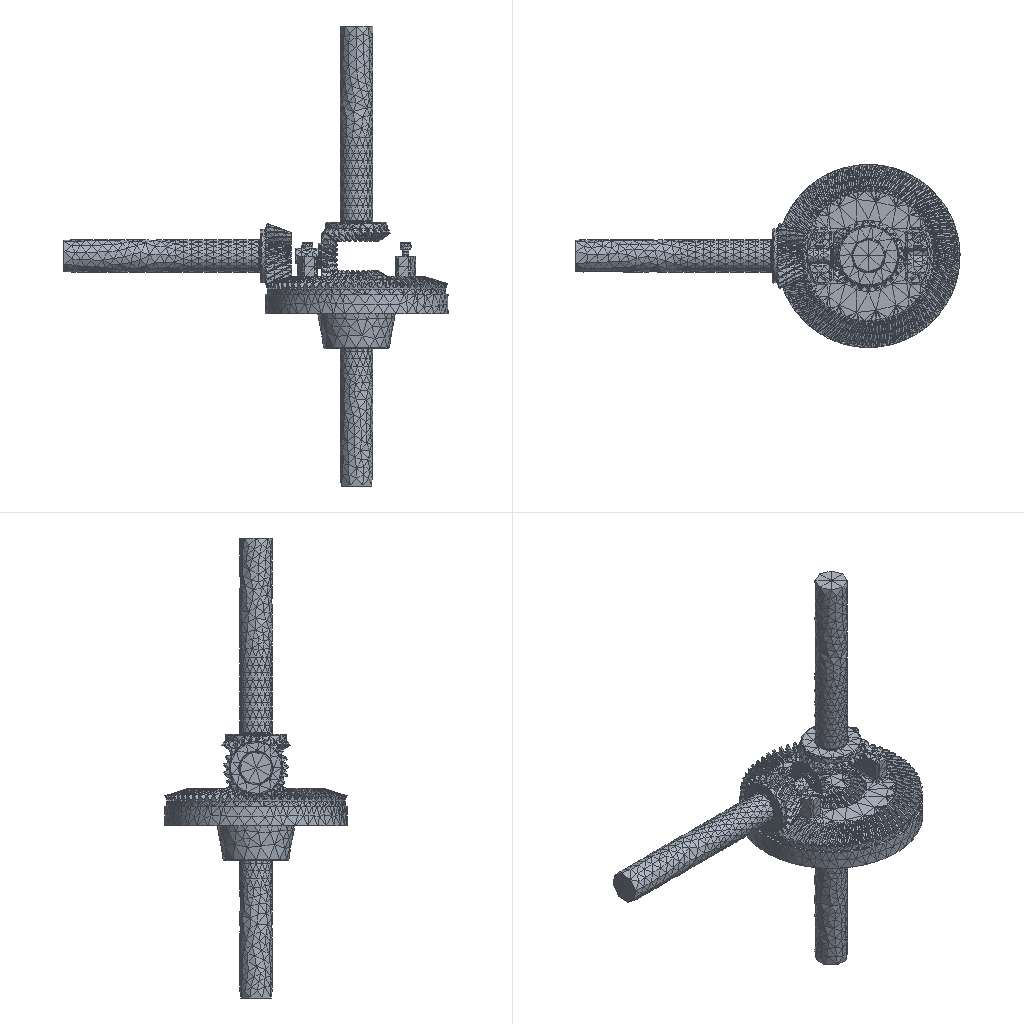Simulation study | ansys workbench
Set-up summary:
category,name,step,type,value,unit,region
solver,ansys_workbench
units,mm-N-s-tonne (MPa),,stated,"/units,MPA"
analysis,LS1,,static
load_step,LS1,LS1,static,nsubst=1; time=1
mesh,nodes,,,47472
mesh,elements,,,28376
element_type,SOLID187,,,25475
element_type,TARGE170,,,1349
element_type,CONTA174,,,1349
element_type,SURF156,,,203
material,Structural Steel,,E,200000,tonne s^-2 mm^-1
material,Structural Steel,,nu,0.3
material,Structural Steel,,density,7.85e-09,tonne mm^-3
material,Structural Steel,,conductivity,60.5,tonne mm s^-3 C^-1
material,Structural Steel,,specific_heat,4.34e+08,mm^2 s^-2 C^-1
material,Structural Steel,,cte,1.2e-05,C^-1
material,Structural Steel,,permeability,10000
material,Structural Steel,,resistivity,0.00017,ohm mm
load,Define Force Using Surface Effect Elements,LS1,surface-effect pres face 1,20.675,,SURF156 #22
bc,Fixed Supports,model,fixed,[dofs=ALL],,_FIXEDSU
contact,Contact Region,,bonded (always),element=CONTA174
contact,Contact Region 2,,bonded (always),element=CONTA174
contact,Contact Region 3,,bonded (always),element=CONTA174
contact,Contact Region 4,,bonded (always),element=CONTA174
contact,Contact Region 5,,bonded (always),element=CONTA174
contact,Contact Region 6,,bonded (always),element=CONTA174
contact,Contact Region 7,,bonded (always),element=CONTA174
named_set,_FIXEDSU,,node,4260
Ansys APDL input file, long lists of numbers shortened:
/batch
/config,noeldb,1     ! force off writing results to database
*get,_wallstrt,active,,time,wall
! ANSYS input file written by Workbench version 2024 R2
! File used for geometry attach:
/title,wbnew--____ (A5)
! ****** Begin Custom Load Command Snippet ******
/COM, ACT Extensions:
/COM,     LSDYNA, 2024.2
/COM,/COM,     ANSYSMotion, 2024.2
/COM,
! ****** End   Custom Load Command Snippet ******
*DIM,_wb_ProjectScratch_dir,string,248
_wb_ProjectScratch_dir(1) = ''
*DIM,_wb_SolverFiles_dir,string,248
_wb_SolverFiles_dir(1) = ''
*DIM,_wb_userfiles_dir,string,248
_wb_userfiles_dir(1) = ''
/com,--- Data in consistent NMM units. See Solving Units in the help system for more information.
/units,MPA
/nopr
/wb,file,start              !  signify a WB generated input file
/prep7
! Turn off shape checking because checks already performed inside WB mesher.
! See help system for more information.
SHPP,OFF,,NOWARN
/nolist
etcon,set             ! allow ANSYS to choose best KEYOP's for 180x elements, resets any applicable keyopt to MAPDL defaults
/com,*********** Nodes for the whole assembly ***********
nblock,3,,52219
(1i9,3e20.9e3)
    15043    -1.469836336E+01     1.140024490E+01     3.492501843E+01
! (47471 more lines like these left out)
-1
/wb,elem,start            !  set before creation of elements
/com,*********** Elements for Body 1 'ISO 4762 M5 x 16' ***********
et,1,187
eblock,19,solid,,1301
(19i9)
        1        1        1        1        0        0        0        0       10        0        1       68      386      103      346      899     1089      894      897
! (2601 more lines like these left out)
-1
/com,*********** Elements for Body 2 'ISO 4762 M5 x 16' ***********
et,2,187
eblock,19,solid,,1301
(19i9)
        2        2        2        2        0        0        0        0       10        0     1302     2441     2759     2476     2719     3272     3462     3267     3270
! (2601 more lines like these left out)
-1
/com,*********** Elements for Body 3 'Bevel Gear1-0' ***********
et,3,187
eblock,19,solid,,2655
(19i9)
        3        3        3        3        0        0        0        0       10        0     2603     4924     5498     5621     5615     6464     9473     6466     6465
! (5309 more lines like these left out)
-1
/com,*********** Elements for Body 4 'Bevel Gear1-0' ***********
et,4,187
eblock,19,solid,,2655
(19i9)
        4        4        4        4        0        0        0        0       10        0     5258    10072    10646    10769    10763    11612    14621    11614    11613
! (5309 more lines like these left out)
-1
/com,*********** Elements for Body 5 'Bevel Gear2-1' ***********
et,5,187
eblock,19,solid,,1087
(19i9)
        5        5        5        5        0        0        0        0       10        0     7913    15249    15257    15436    15420    16410    16446    16418    16416
! (2173 more lines like these left out)
-1
/com,*********** Elements for Body 6 'Bevel Gear1' ***********
et,6,187
eblock,19,solid,,2939
(19i9)
        6        6        6        6        0        0        0        0       10        0     9000    17646    18241    17689    17653    19951    20280    19948    19947
! (5877 more lines like these left out)
-1
/com,*********** Elements for Body 7 'Bevel Gear2' ***********
et,7,187
eblock,19,solid,,13537
(19i9)
        7        7        7        7        0        0        0        0       10        0    11939    24643    26809    26210    26759    37032    45770    37028    37030
! (27073 more lines like these left out)
-1
/wb,elem,end               !  done creating elements
/com,*********** Send User Defined Coordinate System(s) ***********
csys,0
toffst,273.15,      ! Temperature offset from absolute zero
/com,*********** Set Reference Temperature ***********
tref,22.
/wb,mat,start              !  starting to send materials
/com,*********** Send Materials ***********
Temperature = 'TEMP' ! Temperature
MP,DENS,1,7.85e-09,	! tonne mm^-3
MP,ALPX,1,1.2e-05,	! C^-1
MP,C,1,434000000,	! mm^2 s^-2 C^-1
MP,KXX,1,60.5,	! tonne mm s^-3 C^-1
MP,RSVX,1,0.00017,	! ohm mm
MP,EX,1,200000,	! tonne s^-2 mm^-1
MP,NUXY,1,0.3,
MP,MURX,1,10000,
Temperature = 'TEMP' ! Temperature
MP,DENS,2,7.85e-09,	! tonne mm^-3
MP,ALPX,2,1.2e-05,	! C^-1
MP,C,2,434000000,	! mm^2 s^-2 C^-1
MP,KXX,2,60.5,	! tonne mm s^-3 C^-1
MP,RSVX,2,0.00017,	! ohm mm
MP,EX,2,200000,	! tonne s^-2 mm^-1
MP,NUXY,2,0.3,
MP,MURX,2,10000,
Temperature = 'TEMP' ! Temperature
MP,DENS,3,7.85e-09,	! tonne mm^-3
MP,ALPX,3,1.2e-05,	! C^-1
MP,C,3,434000000,	! mm^2 s^-2 C^-1
MP,KXX,3,60.5,	! tonne mm s^-3 C^-1
MP,RSVX,3,0.00017,	! ohm mm
MP,EX,3,200000,	! tonne s^-2 mm^-1
MP,NUXY,3,0.3,
MP,MURX,3,10000,
Temperature = 'TEMP' ! Temperature
MP,DENS,4,7.85e-09,	! tonne mm^-3
MP,ALPX,4,1.2e-05,	! C^-1
MP,C,4,434000000,	! mm^2 s^-2 C^-1
MP,KXX,4,60.5,	! tonne mm s^-3 C^-1
MP,RSVX,4,0.00017,	! ohm mm
MP,EX,4,200000,	! tonne s^-2 mm^-1
MP,NUXY,4,0.3,
MP,MURX,4,10000,
Temperature = 'TEMP' ! Temperature
MP,DENS,5,7.85e-09,	! tonne mm^-3
MP,ALPX,5,1.2e-05,	! C^-1
MP,C,5,434000000,	! mm^2 s^-2 C^-1
MP,KXX,5,60.5,	! tonne mm s^-3 C^-1
MP,RSVX,5,0.00017,	! ohm mm
MP,EX,5,200000,	! tonne s^-2 mm^-1
MP,NUXY,5,0.3,
MP,MURX,5,10000,
Temperature = 'TEMP' ! Temperature
MP,DENS,6,7.85e-09,	! tonne mm^-3
MP,ALPX,6,1.2e-05,	! C^-1
MP,C,6,434000000,	! mm^2 s^-2 C^-1
MP,KXX,6,60.5,	! tonne mm s^-3 C^-1
MP,RSVX,6,0.00017,	! ohm mm
MP,EX,6,200000,	! tonne s^-2 mm^-1
MP,NUXY,6,0.3,
MP,MURX,6,10000,
Temperature = 'TEMP' ! Temperature
MP,DENS,7,7.85e-09,	! tonne mm^-3
MP,ALPX,7,1.2e-05,	! C^-1
MP,C,7,434000000,	! mm^2 s^-2 C^-1
MP,KXX,7,60.5,	! tonne mm s^-3 C^-1
MP,RSVX,7,0.00017,	! ohm mm
MP,EX,7,200000,	! tonne s^-2 mm^-1
MP,NUXY,7,0.3,
MP,MURX,7,10000,
/wb,mat,end                !  done sending materials
!************************* Model Summary ********************
!ISO 4762 M5 x 16,	ç»æé¢,	matid,	1
!ISO 4762 M5 x 16,	ç»æé¢,	matid,	2
!Bevel Gear1-0,	ç»æé¢,	matid,	3
!Bevel Gear1-0,	ç»æé¢,	matid,	4
!Bevel Gear2-1,	ç»æé¢,	matid,	5
!Bevel Gear1,	ç»æé¢,	matid,	6
!Bevel Gear2,	ç»æé¢,	matid,	7
!************************* End Model Summary ********************
! get the diagonal of the bounding box. Needed later for other things
*get,_xmin,node,,mnloc,x
*get,_ymin,node,,mnloc,y
*get,_zmin,node,,mnloc,z
*get,_xmax,node,,mxloc,x
*get,_ymax,node,,mxloc,y
*get,_zmax,node,,mxloc,z
_ASMDIAG=(_xmax-_xmin)*(_xmax-_xmin)+(_ymax-_ymin)*(_ymax-_ymin)+(_zmax-_zmin)*(_zmax-_zmin)
_ASMDIAG=SQRT(_ASMDIAG)
/wb,contact,start          !  starting to send contact
/com,*********** Create Contact "½Ó´¥ÇøÓò" ***********
/com,            Real Constant Set For Above Contact Is 9 & 8
*set,tid,9
*set,cid,8
r,tid
r,cid
et,tid,170
et,cid,174
eblock,10,,,302
(15i9)
    38182        9        9        9        0       37       41       45       45      687      713       45      690
! (301 more lines like these left out)
-1
eblock,10,,,302
(15i9)
    38484        8        8        8        0       37       41       45       45      687      713       45      690
! (301 more lines like these left out)
-1
eblock,10,,,142
(15i9)
    38786        8        9        8        0    24226    24222    25876    25876    34057    34060    25876    34087
! (141 more lines like these left out)
-1
eblock,10,,,142
(15i9)
    38928        9        8        9        0    24226    24222    25876    25876    34057    34060    25876    34087
! (141 more lines like these left out)
-1
keyo,cid,8,2               ! auto create asymmetric contact (from Program Controlled setting)
keyo,cid,10,0              ! adjust contact stiffness each NR iteration (from Program Controlled setting)
keyo,cid,12,5              ! bonded always
keyo,cid,18,1              ! small sliding turned on by application
keyo,cid,2,2               ! MPC for bonded contacts (from Program Controlled setting)
keyo,tid,5,0               ! Automatic constraint type detection
keyo,cid,4,2               ! on nodal point - normal to target surface (from Program Controlled setting)
keyo,cid,9,1               ! ignore initial gaps/penetration
keyo,cid,7,0               ! No Prediction
rmod,tid,3,10.      ! FKN
rmod,tid,5,0.       ! ICONT
rmod,tid,6,0.       ! PINB
rmod,tid,10,0.      ! CNOF
rmod,tid,12,0.      ! FKT
rmod,tid,36,44      ! WB DSID
rmod,cid,3,10.      ! FKN
rmod,cid,5,0.       ! ICONT
rmod,cid,6,0.       ! PINB
rmod,cid,10,0.      ! CNOF
rmod,cid,12,0.      ! FKT
rmod,cid,36,44      ! WB DSID
/com,*********** Create Contact "½Ó´¥ÇøÓò 2" ***********
/com,            Real Constant Set For Above Contact Is 11 & 10
*set,tid,11
*set,cid,10
r,tid
r,cid
et,tid,170
et,cid,174
eblock,10,,,302
(15i9)
    39070       11       11       11        0     2410     2414     2418     2418     3060     3086     2418     3063
! (301 more lines like these left out)
-1
eblock,10,,,302
(15i9)
    39372       10       10       10        0     2410     2414     2418     2418     3060     3086     2418     3063
! (301 more lines like these left out)
-1
eblock,10,,,136
(15i9)
    39674       10       11       10        0    24050    24057    25987    25987    32541    32591    25987    32544
! (135 more lines like these left out)
-1
eblock,10,,,136
(15i9)
    39810       11       10       11        0    24050    24057    25987    25987    32541    32591    25987    32544
! (135 more lines like these left out)
-1
keyo,cid,8,2               ! auto create asymmetric contact (from Program Controlled setting)
keyo,cid,10,0              ! adjust contact stiffness each NR iteration (from Program Controlled setting)
keyo,cid,12,5              ! bonded always
keyo,cid,18,1              ! small sliding turned on by application
keyo,cid,2,2               ! MPC for bonded contacts (from Program Controlled setting)
keyo,tid,5,0               ! Automatic constraint type detection
keyo,cid,4,2               ! on nodal point - normal to target surface (from Program Controlled setting)
keyo,cid,9,1               ! ignore initial gaps/penetration
keyo,cid,7,0               ! No Prediction
rmod,tid,3,10.      ! FKN
rmod,tid,5,0.       ! ICONT
rmod,tid,6,0.       ! PINB
rmod,tid,10,0.      ! CNOF
rmod,tid,12,0.      ! FKT
rmod,tid,36,47      ! WB DSID
rmod,cid,3,10.      ! FKN
rmod,cid,5,0.       ! ICONT
rmod,cid,6,0.       ! PINB
rmod,cid,10,0.      ! CNOF
rmod,cid,12,0.      ! FKT
rmod,cid,36,47      ! WB DSID
/com,*********** Create Contact "½Ó´¥ÇøÓò 3" ***********
/com,            Real Constant Set For Above Contact Is 13 & 12
*set,tid,13
*set,cid,12
r,tid
r,cid
et,tid,170
et,cid,174
eblock,10,,,44
(15i9)
    39946       13       13       13        0     4939     4944     4941     4941     6536     6546     4941     6534
! (43 more lines like these left out)
-1
eblock,10,,,44
(15i9)
    39990       12       12       12        0     4939     4944     4941     4941     6536     6546     4941     6534
! (43 more lines like these left out)
-1
eblock,10,,,44
(15i9)
    40034       12       13       12        0    15189    15192    15188    15188    16126    16123    15188    16121
! (43 more lines like these left out)
-1
eblock,10,,,44
(15i9)
    40078       13       12       13        0    15189    15192    15188    15188    16126    16123    15188    16121
! (43 more lines like these left out)
-1
keyo,cid,8,2               ! auto create asymmetric contact (from Program Controlled setting)
keyo,cid,10,0              ! adjust contact stiffness each NR iteration (from Program Controlled setting)
keyo,cid,12,5              ! bonded always
keyo,cid,18,1              ! small sliding turned on by application
keyo,cid,2,2               ! MPC for bonded contacts (from Program Controlled setting)
keyo,tid,5,0               ! Automatic constraint type detection
keyo,cid,4,2               ! on nodal point - normal to target surface (from Program Controlled setting)
keyo,cid,9,1               ! ignore initial gaps/penetration
keyo,cid,7,0               ! No Prediction
rmod,tid,3,10.      ! FKN
rmod,tid,5,0.       ! ICONT
rmod,tid,6,0.       ! PINB
rmod,tid,10,0.      ! CNOF
rmod,tid,12,0.      ! FKT
rmod,tid,36,50      ! WB DSID
rmod,cid,3,10.      ! FKN
rmod,cid,5,0.       ! ICONT
rmod,cid,6,0.       ! PINB
rmod,cid,10,0.      ! CNOF
rmod,cid,12,0.      ! FKT
rmod,cid,36,50      ! WB DSID
/com,*********** Create Contact "½Ó´¥ÇøÓò 4" ***********
/com,            Real Constant Set For Above Contact Is 15 & 14
*set,tid,15
*set,cid,14
r,tid
r,cid
et,tid,170
et,cid,174
eblock,10,,,87
(15i9)
    40122       15       15       15        0     5075     5101     5076     5076     7236     7243     5076     7234
! (86 more lines like these left out)
-1
eblock,10,,,87
(15i9)
    40209       14       14       14        0     5075     5101     5076     5076     7236     7243     5076     7234
! (86 more lines like these left out)
-1
eblock,10,,,29
(15i9)
    40296       14       15       14        0    24126    24808    24127    24127    33136    33149    24127    33135
! (28 more lines like these left out)
-1
eblock,10,,,29
(15i9)
    40325       15       14       15        0    24126    24808    24127    24127    33136    33149    24127    33135
! (28 more lines like these left out)
-1
keyo,cid,8,2               ! auto create asymmetric contact (from Program Controlled setting)
keyo,cid,10,0              ! adjust contact stiffness each NR iteration (from Program Controlled setting)
keyo,cid,12,5              ! bonded always
keyo,cid,18,1              ! small sliding turned on by application
keyo,cid,2,2               ! MPC for bonded contacts (from Program Controlled setting)
keyo,tid,5,0               ! Automatic constraint type detection
keyo,cid,4,2               ! on nodal point - normal to target surface (from Program Controlled setting)
keyo,cid,9,1               ! ignore initial gaps/penetration
keyo,cid,7,0               ! No Prediction
rmod,tid,3,10.      ! FKN
rmod,tid,5,0.       ! ICONT
rmod,tid,6,0.       ! PINB
rmod,tid,10,0.      ! CNOF
rmod,tid,12,0.      ! FKT
rmod,tid,36,53      ! WB DSID
rmod,cid,3,10.      ! FKN
rmod,cid,5,0.       ! ICONT
rmod,cid,6,0.       ! PINB
rmod,cid,10,0.      ! CNOF
rmod,cid,12,0.      ! FKT
rmod,cid,36,53      ! WB DSID
/com,*********** Create Contact "½Ó´¥ÇøÓò 5" ***********
/com,            Real Constant Set For Above Contact Is 17 & 16
*set,tid,17
*set,cid,16
r,tid
r,cid
et,tid,170
et,cid,174
eblock,10,,,40
(15i9)
    40354       17       17       17        0    10063    10068    10065    10065    11568    11578    10065    11566
! (39 more lines like these left out)
-1
eblock,10,,,40
(15i9)
    40394       16       16       16        0    10063    10068    10065    10065    11568    11578    10065    11566
! (39 more lines like these left out)
-1
eblock,10,,,40
(15i9)
    40434       16       17       16        0    15069    15072    15068    15068    15579    15576    15068    15574
! (39 more lines like these left out)
-1
eblock,10,,,40
(15i9)
    40474       17       16       17        0    15069    15072    15068    15068    15579    15576    15068    15574
! (39 more lines like these left out)
-1
keyo,cid,8,2               ! auto create asymmetric contact (from Program Controlled setting)
keyo,cid,10,0              ! adjust contact stiffness each NR iteration (from Program Controlled setting)
keyo,cid,12,5              ! bonded always
keyo,cid,18,1              ! small sliding turned on by application
keyo,cid,2,2               ! MPC for bonded contacts (from Program Controlled setting)
keyo,tid,5,0               ! Automatic constraint type detection
keyo,cid,4,2               ! on nodal point - normal to target surface (from Program Controlled setting)
keyo,cid,9,1               ! ignore initial gaps/penetration
keyo,cid,7,0               ! No Prediction
rmod,tid,3,10.      ! FKN
rmod,tid,5,0.       ! ICONT
rmod,tid,6,0.       ! PINB
rmod,tid,10,0.      ! CNOF
rmod,tid,12,0.      ! FKT
rmod,tid,36,56      ! WB DSID
rmod,cid,3,10.      ! FKN
rmod,cid,5,0.       ! ICONT
rmod,cid,6,0.       ! PINB
rmod,cid,10,0.      ! CNOF
rmod,cid,12,0.      ! FKT
rmod,cid,36,56      ! WB DSID
/com,*********** Create Contact "½Ó´¥ÇøÓò 6" ***********
/com,            Real Constant Set For Above Contact Is 19 & 18
*set,tid,19
*set,cid,18
r,tid
r,cid
et,tid,170
et,cid,174
eblock,10,,,103
(15i9)
    40514       19       19       19        0    15271    15275    15380    15380    16506    16529    15380    16509
! (102 more lines like these left out)
-1
eblock,10,,,103
(15i9)
    40617       18       18       18        0    15271    15275    15380    15380    16506    16529    15380    16509
! (102 more lines like these left out)
-1
eblock,10,,,32
(15i9)
    40720       18       19       18        0    24182    24062    26860    26860    32625    32626    26860    33754
! (31 more lines like these left out)
-1
eblock,10,,,32
(15i9)
    40752       19       18       19        0    24182    24062    26860    26860    32625    32626    26860    33754
! (31 more lines like these left out)
-1
keyo,cid,8,2               ! auto create asymmetric contact (from Program Controlled setting)
keyo,cid,10,0              ! adjust contact stiffness each NR iteration (from Program Controlled setting)
keyo,cid,12,5              ! bonded always
keyo,cid,18,1              ! small sliding turned on by application
keyo,cid,2,0               ! augmented Lagrange (from Program Controlled setting)
keyo,cid,4,0               ! on Gauss point (from Program Controlled setting)
keyo,cid,9,1               ! ignore initial gaps/penetration
keyo,cid,7,0               ! No Prediction
rmod,tid,3,10.      ! FKN
rmod,tid,5,0.       ! ICONT
rmod,tid,6,0.       ! PINB
rmod,tid,10,0.      ! CNOF
rmod,tid,12,0.      ! FKT
rmod,tid,36,59      ! WB DSID
rmod,cid,3,10.      ! FKN
rmod,cid,5,0.       ! ICONT
rmod,cid,6,0.       ! PINB
rmod,cid,10,0.      ! CNOF
rmod,cid,12,0.      ! FKT
rmod,cid,36,59      ! WB DSID
/com,*********** Create Contact "½Ó´¥ÇøÓò 7" ***********
/com,            Real Constant Set For Above Contact Is 21 & 20
*set,tid,21
*set,cid,20
r,tid
r,cid
et,tid,170
et,cid,174
eblock,10,,,24
(15i9)
    40784       21       21       21        0    17568    17566    17575    17575    19577    19579    17575    19586
! (23 more lines like these left out)
-1
eblock,10,,,24
(15i9)
    40808       20       20       20        0    17568    17566    17575    17575    19577    19579    17575    19586
! (23 more lines like these left out)
-1
eblock,10,,,24
(15i9)
    40832       20       21       20        0    22946    22949    22952    22952    26874    26893    22952    26875
! (23 more lines like these left out)
-1
eblock,10,,,24
(15i9)
    40856       21       20       21        0    22946    22949    22952    22952    26874    26893    22952    26875
! (23 more lines like these left out)
-1
keyo,cid,8,2               ! auto create asymmetric contact (from Program Controlled setting)
keyo,cid,10,0              ! adjust contact stiffness each NR iteration (from Program Controlled setting)
keyo,cid,12,5              ! bonded always
keyo,cid,18,1              ! small sliding turned on by application
keyo,cid,2,2               ! MPC for bonded contacts (from Program Controlled setting)
keyo,tid,5,0               ! Automatic constraint type detection
keyo,cid,4,2               ! on nodal point - normal to target surface (from Program Controlled setting)
keyo,cid,9,1               ! ignore initial gaps/penetration
keyo,cid,7,0               ! No Prediction
rmod,tid,3,10.      ! FKN
rmod,tid,5,0.       ! ICONT
rmod,tid,6,0.       ! PINB
rmod,tid,10,0.      ! CNOF
rmod,tid,12,0.      ! FKT
rmod,tid,36,62      ! WB DSID
rmod,cid,3,10.      ! FKN
rmod,cid,5,0.       ! ICONT
rmod,cid,6,0.       ! PINB
rmod,cid,10,0.      ! CNOF
rmod,cid,12,0.      ! FKT
rmod,cid,36,62      ! WB DSID
nsel,all
esel,all
/wb,contact,end            !  done creating contacts
/golist
/wb,load,start             !  starting to send loads
/com,*********** Fixed Supports ***********
CMBLOCK,_FIXEDSU,NODE,     4260
(8i10)
      5047      5048      5049      5050      5051      5052      5053      5054
! (532 more lines like these left out)
cmsel,s,_FIXEDSU
d,all,all
nsel,all
/com,*********** Define Force Using Surface Effect Elements ***********
local,12,0,0.,0.,0.,0.,0.,0.
csys,0
et,22,156
mat,22
keyop,22,5,1        !  No orientation node
eblock,10,,,203
(15i9)
    40880       22       22       22       12    17322    17324    18412
! (202 more lines like these left out)
-1
esel,s,type,,22
keyop,22,2,1        ! Apply load in local coordinate system
keyop,22,7,1        ! Use original area so load is constant in large deformation
esel,all
/gst,on,on
fini
*get,_numnode,node,0,count
*get,_numelem,elem,0,count
*get, _MAXELEMNUM, elem, 0, NUM, MAX
*get, _MAXNODENUM, node, 0, NUM, MAX
*get, _MAXELEMTYPE, etyp, 0, NUM, MAX
*get, _MAXREALCONST, rcon, 0, NUM, MAX
/go
/wb,load,end               !  done creating loads
/com,--- Number of total nodes = %_numnode%
/com,--- Number of contact elements = 2901
/com,--- Number of spring elements = 0
/com,--- Number of bearing elements = 0
/com,--- Number of solid elements = 25475
/com,--- Number of condensed parts = 0
/com,--- Number of total elements = %_numelem%
*get,_wallbsol,active,,time,wall
/com,****************************************************************************
/com,*************************    SOLUTION       ********************************
/com,****************************************************************************
/solu
antype,0                   ! static analysis
_thickRatio=  1     ! Ratio of thick parts in the model
eqsl,pcg,1e-8,,,,,,1
cntr,print,1               ! print out contact info and also make no initial contact an error
dmpoption,emat,no             ! Don't combine emat file for DANSYS
dmpoption,esav,no             ! Don't combine esav file for DANSYS
nldiag,cont,iter           ! print out contact info each equilibrium iteration
rescontrol,,none                 ! Do not keep any restart files
/com,****************************************************
/com,******************* SOLVE FOR LS 1 OF 1 ****************
esel,s,type,,22
nsle
sfe,all,1,pres,1,20.675
sfe,all,2,pres,1,0.
sfe,all,3,pres,1,0.
nsel,all
esel,all
/nopr
/gopr
nsub,1,1,1
time,1.
outres,erase
outres,all,none
outres,nsol,all,
outres,rsol,all
outres,eangl,all
outres,etmp,all
outres,veng,all
outres,strs,all,
outres,epel,all,
outres,eppl,all,
outres,cont,all,
! *********** WB SOLVE COMMAND ***********
! check interactive state
*get,ANSINTER_,active,,int
*if,ANSINTER_,ne,0,then
/eof
*endif
solve
/com *************** Write FE CONNECTORS *********
CEWRITE,file,ce,,INTE
/com,****************************************************
/com,*************** FINISHED SOLVE FOR LS 1 *************
*get,_wallasol,active,,time,wall
/nopr
*get,_numnode,node,0,count
*get,_numelem,elem,0,count
*get, _MAXELEMNUM, elem, 0, NUM, MAX
*get, _MAXNODENUM, node, 0, NUM, MAX,,,INTERNAL
*get, _MAXELEMTYPE, etyp, 0, NUM, MAX
*get, _MAXREALCONST, rcon, 0, NUM, MAX
*get,_NSOLTHREADS,active,0,ntfs
*get,_NSOLPROCESSES,active,0,npfs
/gopr
*get,_PCGITER,active,,solu,cgiter
/post1
xmlo,ENCODING,ISO-8859-1
xmlo,parm
/xml,parm,xml
fini
/gopr
*get,_walldone,active,,time,wall
_preptime=(_wallbsol-_wallstrt)*3600
_solvtime=(_wallasol-_wallbsol)*3600
_posttime=(_walldone-_wallasol)*3600
_totaltim=(_walldone-_wallstrt)*3600
*get,_dlbratio,active,0,solu,dlbr
*get,_combtime,active,0,solu,comb
*get,_ssmode,active,0,solu,ssmm
*get,_ndofs,active,0,solu,ndof
*get,_sol_end_time,active,0,set,time
*if,_sol_end_time,eq,1.,then
/fclean				!clean distributed files
*endif
/com,--- Total number of nodes = %_numnode%
/com,--- Total number of elements = %_numelem%
/com,--- Element load balance ratio = %_dlbratio%
/com,--- Time to combine distributed files = %_combtime%
/com,--- Sparse memory mode = %_ssmode%
/com,--- Number of DOF = %_ndofs%
/wb,file,end               ! done with WB generated input
Results summary:
result,analyses[0].index,,,1
result,analyses[0].system,,,SYS
result,analyses[0].deck,,,deck.dat
result,analyses[0].solve_status,,,completed
result,analyses[0].analysis_type,,,static
result,analyses[0].physics,,,mechanical
result,analyses[0].unit_system,,,"NMM: mm, ton, N, s, mV, mA, degC"
result,analyses[0].n_sets,,,1
result,analyses[0].load_steps[0].set,set=1,,1
result,analyses[0].load_steps[0].time_or_freq,set=1,,1
result,analyses[0].load_steps[0].max_displacement_magnitude,set=1,,0.04091
result,analyses[0].load_steps[0].max_von_mises_nodal,set=1,,283.48
result,analyses[0].load_steps[0].reaction_force_sum_xyz[1],set=1,,-29999.9
result,analyses[0].load_steps[0].reaction_force_sum_xyz[2],set=1,,-8.16175e-06
result,analyses[0].load_steps[0].reaction_force_sum_xyz[3],set=1,,-1.63293e-05